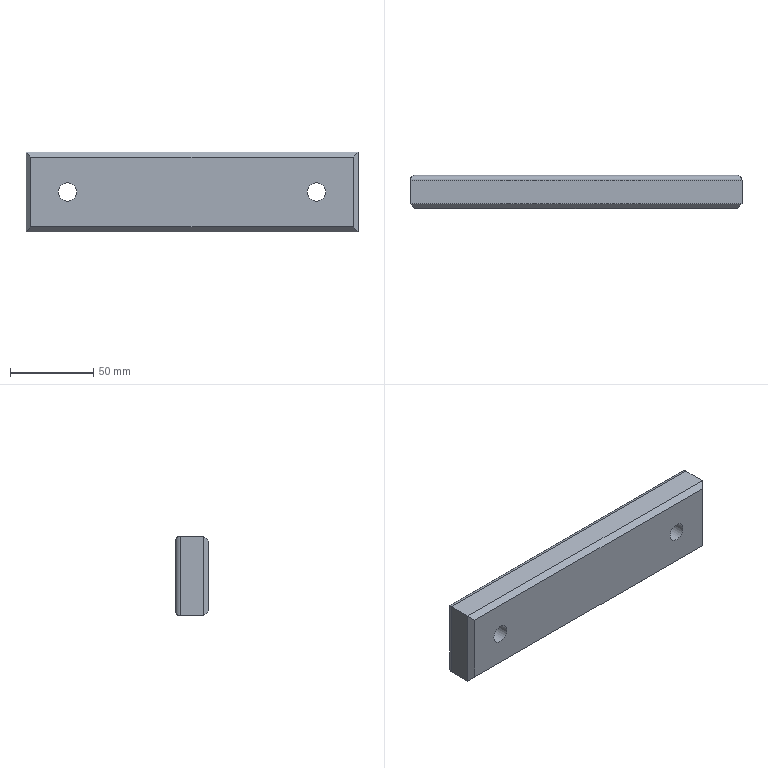Part | NX | features MAIN_BODY 2 | 1 solid | 20 faces | box 200 x 20 x 48 mm | volume 181563 mm3 | plane 12 | cylinder 8 | commonest cylinder face diameters 6 x4 11 x2 17.5 x2
STEP:
#1=CARTESIAN_POINT('',(95.,343.,-345.));
#2=VERTEX_POINT('',#1);
#3=CARTESIAN_POINT('',(95.,357.,-345.));
#4=VERTEX_POINT('',#3);
#5=CARTESIAN_POINT('',(95.,340.,-345.));
#6=DIRECTION('',(0.,1.,0.));
#7=VECTOR('',#6,1000.);
#8=LINE('',#5,#7);
#9=EDGE_CURVE('',#2,#4,#8,.T.);
#10=ORIENTED_EDGE('',*,*,#9,.F.);
#11=CARTESIAN_POINT('',(95.,343.,-297.));
#12=VERTEX_POINT('',#11);
#13=CARTESIAN_POINT('',(95.,343.,-297.));
#14=DIRECTION('',(0.,0.,1.));
#15=VECTOR('',#14,1000.);
#16=LINE('',#13,#15);
#17=EDGE_CURVE('',#2,#12,#16,.T.);
#18=ORIENTED_EDGE('',*,*,#17,.T.);
#19=CARTESIAN_POINT('',(95.,357.,-297.));
#20=VERTEX_POINT('',#19);
#21=CARTESIAN_POINT('',(95.,340.,-297.));
#22=DIRECTION('',(0.,1.,0.));
#23=VECTOR('',#22,1000.);
#24=LINE('',#21,#23);
#25=EDGE_CURVE('',#12,#20,#24,.T.);
#26=ORIENTED_EDGE('',*,*,#25,.T.);
#27=CARTESIAN_POINT('',(95.,357.,-297.));
#28=DIRECTION('',(0.,0.,-1.));
#29=VECTOR('',#28,1000.);
#30=LINE('',#27,#29);
#31=EDGE_CURVE('',#20,#4,#30,.T.);
#32=ORIENTED_EDGE('',*,*,#31,.T.);
#33=EDGE_LOOP('',(#10,#18,#26,#32));
#34=FACE_BOUND('',#33,.T.);
#35=CARTESIAN_POINT('',(95.,340.,-297.));
#36=DIRECTION('',(1.,0.,0.));
#37=DIRECTION('',(0.,1.,0.));
#38=AXIS2_PLACEMENT_3D('',#35,#36,#37);
#39=PLANE('',#38);
#40=ADVANCED_FACE('',(#34),#39,.F.);
#41=CARTESIAN_POINT('',(295.,343.,-345.));
#42=VERTEX_POINT('',#41);
#43=CARTESIAN_POINT('',(295.,357.,-345.));
#44=VERTEX_POINT('',#43);
#45=CARTESIAN_POINT('',(295.,340.,-345.));
#46=DIRECTION('',(0.,1.,0.));
#47=VECTOR('',#46,1000.);
#48=LINE('',#45,#47);
#49=EDGE_CURVE('',#42,#44,#48,.T.);
#50=ORIENTED_EDGE('',*,*,#49,.F.);
#51=CARTESIAN_POINT('',(95.,343.,-345.));
#52=DIRECTION('',(-1.,0.,0.));
#53=VECTOR('',#52,1000.);
#54=LINE('',#51,#53);
#55=EDGE_CURVE('',#42,#2,#54,.T.);
#56=ORIENTED_EDGE('',*,*,#55,.T.);
#57=ORIENTED_EDGE('',*,*,#9,.T.);
#58=CARTESIAN_POINT('',(95.,357.,-345.));
#59=DIRECTION('',(1.,0.,0.));
#60=VECTOR('',#59,1000.);
#61=LINE('',#58,#60);
#62=EDGE_CURVE('',#4,#44,#61,.T.);
#63=ORIENTED_EDGE('',*,*,#62,.T.);
#64=EDGE_LOOP('',(#50,#56,#57,#63));
#65=FACE_BOUND('',#64,.T.);
#66=CARTESIAN_POINT('',(95.,340.,-345.));
#67=DIRECTION('',(0.,0.,1.));
#68=DIRECTION('',(-1.,0.,0.));
#69=AXIS2_PLACEMENT_3D('',#66,#67,#68);
#70=PLANE('',#69);
#71=ADVANCED_FACE('',(#65),#70,.F.);
#72=CARTESIAN_POINT('',(295.,343.,-297.));
#73=VERTEX_POINT('',#72);
#74=CARTESIAN_POINT('',(295.,357.,-297.));
#75=VERTEX_POINT('',#74);
#76=CARTESIAN_POINT('',(295.,340.,-297.));
#77=DIRECTION('',(0.,1.,0.));
#78=VECTOR('',#77,1000.);
#79=LINE('',#76,#78);
#80=EDGE_CURVE('',#73,#75,#79,.T.);
#81=ORIENTED_EDGE('',*,*,#80,.F.);
#82=CARTESIAN_POINT('',(295.,343.,-345.));
#83=DIRECTION('',(0.,0.,-1.));
#84=VECTOR('',#83,1000.);
#85=LINE('',#82,#84);
#86=EDGE_CURVE('',#73,#42,#85,.T.);
#87=ORIENTED_EDGE('',*,*,#86,.T.);
#88=ORIENTED_EDGE('',*,*,#49,.T.);
#89=CARTESIAN_POINT('',(295.,357.,-345.));
#90=DIRECTION('',(0.,0.,1.));
#91=VECTOR('',#90,1000.);
#92=LINE('',#89,#91);
#93=EDGE_CURVE('',#44,#75,#92,.T.);
#94=ORIENTED_EDGE('',*,*,#93,.T.);
#95=EDGE_LOOP('',(#81,#87,#88,#94));
#96=FACE_BOUND('',#95,.T.);
#97=CARTESIAN_POINT('',(295.,340.,-345.));
#98=DIRECTION('',(-1.,0.,0.));
#99=DIRECTION('',(0.,-1.,0.));
#100=AXIS2_PLACEMENT_3D('',#97,#98,#99);
#101=PLANE('',#100);
#102=ADVANCED_FACE('',(#96),#101,.F.);
#103=ORIENTED_EDGE('',*,*,#25,.F.);
#104=CARTESIAN_POINT('',(295.,343.,-297.));
#105=DIRECTION('',(1.,0.,0.));
#106=VECTOR('',#105,1000.);
#107=LINE('',#104,#106);
#108=EDGE_CURVE('',#12,#73,#107,.T.);
#109=ORIENTED_EDGE('',*,*,#108,.T.);
#110=ORIENTED_EDGE('',*,*,#80,.T.);
#111=CARTESIAN_POINT('',(295.,357.,-297.));
#112=DIRECTION('',(-1.,0.,0.));
#113=VECTOR('',#112,1000.);
#114=LINE('',#111,#113);
#115=EDGE_CURVE('',#75,#20,#114,.T.);
#116=ORIENTED_EDGE('',*,*,#115,.T.);
#117=EDGE_LOOP('',(#103,#109,#110,#116));
#118=FACE_BOUND('',#117,.T.);
#119=CARTESIAN_POINT('',(295.,340.,-297.));
#120=DIRECTION('',(0.,0.,-1.));
#121=DIRECTION('',(1.,0.,0.));
#122=AXIS2_PLACEMENT_3D('',#119,#120,#121);
#123=PLANE('',#122);
#124=ADVANCED_FACE('',(#118),#123,.F.);
#125=CARTESIAN_POINT('',(98.,340.,-342.));
#126=VERTEX_POINT('',#125);
#127=CARTESIAN_POINT('',(292.,340.,-342.));
#128=VERTEX_POINT('',#127);
#129=CARTESIAN_POINT('',(295.,340.,-342.));
#130=DIRECTION('',(1.,0.,0.));
#131=VECTOR('',#130,1000.);
#132=LINE('',#129,#131);
#133=EDGE_CURVE('',#126,#128,#132,.T.);
#134=ORIENTED_EDGE('',*,*,#133,.T.);
#135=CARTESIAN_POINT('',(292.,340.,-300.));
#136=VERTEX_POINT('',#135);
#137=CARTESIAN_POINT('',(292.,340.,-297.));
#138=DIRECTION('',(0.,0.,1.));
#139=VECTOR('',#138,1000.);
#140=LINE('',#137,#139);
#141=EDGE_CURVE('',#128,#136,#140,.T.);
#142=ORIENTED_EDGE('',*,*,#141,.T.);
#143=CARTESIAN_POINT('',(98.,340.,-300.));
#144=VERTEX_POINT('',#143);
#145=CARTESIAN_POINT('',(95.,340.,-300.));
#146=DIRECTION('',(-1.,0.,0.));
#147=VECTOR('',#146,1000.);
#148=LINE('',#145,#147);
#149=EDGE_CURVE('',#136,#144,#148,.T.);
#150=ORIENTED_EDGE('',*,*,#149,.T.);
#151=CARTESIAN_POINT('',(98.,340.,-345.));
#152=DIRECTION('',(0.,0.,-1.));
#153=VECTOR('',#152,1000.);
#154=LINE('',#151,#153);
#155=EDGE_CURVE('',#144,#126,#154,.T.);
#156=ORIENTED_EDGE('',*,*,#155,.T.);
#157=EDGE_LOOP('',(#134,#142,#150,#156));
#158=FACE_BOUND('',#157,.T.);
#159=CARTESIAN_POINT('',(275.5,340.,-321.));
#160=VERTEX_POINT('',#159);
#161=CARTESIAN_POINT('',(270.,340.,-321.));
#162=DIRECTION('',(0.,-1.,0.));
#163=DIRECTION('',(1.,0.,0.));
#164=AXIS2_PLACEMENT_3D('',#161,#162,#163);
#165=CIRCLE('',#164,5.5);
#166=EDGE_CURVE('',#160,#160,#165,.T.);
#167=ORIENTED_EDGE('',*,*,#166,.F.);
#168=EDGE_LOOP('',(#167));
#169=FACE_BOUND('',#168,.T.);
#170=CARTESIAN_POINT('',(125.5,340.,-321.));
#171=VERTEX_POINT('',#170);
#172=CARTESIAN_POINT('',(120.,340.,-321.));
#173=DIRECTION('',(0.,-1.,0.));
#174=DIRECTION('',(1.,0.,0.));
#175=AXIS2_PLACEMENT_3D('',#172,#173,#174);
#176=CIRCLE('',#175,5.5);
#177=EDGE_CURVE('',#171,#171,#176,.T.);
#178=ORIENTED_EDGE('',*,*,#177,.F.);
#179=EDGE_LOOP('',(#178));
#180=FACE_BOUND('',#179,.T.);
#181=CARTESIAN_POINT('',(95.,340.,-345.));
#182=DIRECTION('',(0.,-1.,0.));
#183=DIRECTION('',(1.,0.,0.));
#184=AXIS2_PLACEMENT_3D('',#181,#182,#183);
#185=PLANE('',#184);
#186=ADVANCED_FACE('',(#158,#169,#180),#185,.T.);
#187=CARTESIAN_POINT('',(98.,360.,-342.));
#188=VERTEX_POINT('',#187);
#189=CARTESIAN_POINT('',(98.,360.,-300.));
#190=VERTEX_POINT('',#189);
#191=CARTESIAN_POINT('',(98.,360.,-345.));
#192=DIRECTION('',(0.,0.,-1.));
#193=VECTOR('',#192,1000.);
#194=LINE('',#191,#193);
#195=EDGE_CURVE('',#188,#190,#194,.F.);
#196=ORIENTED_EDGE('',*,*,#195,.T.);
#197=CARTESIAN_POINT('',(292.,360.,-300.));
#198=VERTEX_POINT('',#197);
#199=CARTESIAN_POINT('',(95.,360.,-300.));
#200=DIRECTION('',(-1.,0.,0.));
#201=VECTOR('',#200,1000.);
#202=LINE('',#199,#201);
#203=EDGE_CURVE('',#190,#198,#202,.F.);
#204=ORIENTED_EDGE('',*,*,#203,.T.);
#205=CARTESIAN_POINT('',(292.,360.,-342.));
#206=VERTEX_POINT('',#205);
#207=CARTESIAN_POINT('',(292.,360.,-345.));
#208=DIRECTION('',(0.,0.,1.));
#209=VECTOR('',#208,1000.);
#210=LINE('',#207,#209);
#211=EDGE_CURVE('',#198,#206,#210,.F.);
#212=ORIENTED_EDGE('',*,*,#211,.T.);
#213=CARTESIAN_POINT('',(95.,360.,-342.));
#214=DIRECTION('',(1.,0.,0.));
#215=VECTOR('',#214,1000.);
#216=LINE('',#213,#215);
#217=EDGE_CURVE('',#206,#188,#216,.F.);
#218=ORIENTED_EDGE('',*,*,#217,.T.);
#219=EDGE_LOOP('',(#196,#204,#212,#218));
#220=FACE_BOUND('',#219,.T.);
#221=CARTESIAN_POINT('',(278.75,360.,-321.));
#222=VERTEX_POINT('',#221);
#223=CARTESIAN_POINT('',(270.,360.,-321.));
#224=DIRECTION('',(0.,-1.,0.));
#225=DIRECTION('',(1.,0.,0.));
#226=AXIS2_PLACEMENT_3D('',#223,#224,#225);
#227=CIRCLE('',#226,8.75);
#228=EDGE_CURVE('',#222,#222,#227,.T.);
#229=ORIENTED_EDGE('',*,*,#228,.T.);
#230=EDGE_LOOP('',(#229));
#231=FACE_BOUND('',#230,.T.);
#232=CARTESIAN_POINT('',(128.75,360.,-321.));
#233=VERTEX_POINT('',#232);
#234=CARTESIAN_POINT('',(120.,360.,-321.));
#235=DIRECTION('',(0.,-1.,0.));
#236=DIRECTION('',(1.,0.,0.));
#237=AXIS2_PLACEMENT_3D('',#234,#235,#236);
#238=CIRCLE('',#237,8.75);
#239=EDGE_CURVE('',#233,#233,#238,.T.);
#240=ORIENTED_EDGE('',*,*,#239,.T.);
#241=EDGE_LOOP('',(#240));
#242=FACE_BOUND('',#241,.T.);
#243=CARTESIAN_POINT('',(95.,360.,-345.));
#244=DIRECTION('',(0.,-1.,0.));
#245=DIRECTION('',(1.,0.,0.));
#246=AXIS2_PLACEMENT_3D('',#243,#244,#245);
#247=PLANE('',#246);
#248=ADVANCED_FACE('',(#220,#231,#242),#247,.F.);
#249=ORIENTED_EDGE('',*,*,#177,.T.);
#250=EDGE_LOOP('',(#249));
#251=FACE_BOUND('',#250,.T.);
#252=CARTESIAN_POINT('',(125.5,348.,-321.));
#253=VERTEX_POINT('',#252);
#254=CARTESIAN_POINT('',(120.,348.,-321.));
#255=DIRECTION('',(0.,-1.,0.));
#256=DIRECTION('',(1.,0.,0.));
#257=AXIS2_PLACEMENT_3D('',#254,#255,#256);
#258=CIRCLE('',#257,5.5);
#259=EDGE_CURVE('',#253,#253,#258,.T.);
#260=ORIENTED_EDGE('',*,*,#259,.F.);
#261=EDGE_LOOP('',(#260));
#262=FACE_BOUND('',#261,.T.);
#263=CARTESIAN_POINT('',(120.,310.,-321.));
#264=DIRECTION('',(0.,-1.,0.));
#265=DIRECTION('',(1.,0.,0.));
#266=AXIS2_PLACEMENT_3D('',#263,#264,#265);
#267=CYLINDRICAL_SURFACE('',#266,5.5);
#268=ADVANCED_FACE('',(#251,#262),#267,.F.);
#269=ORIENTED_EDGE('',*,*,#259,.T.);
#270=EDGE_LOOP('',(#269));
#271=FACE_BOUND('',#270,.T.);
#272=CARTESIAN_POINT('',(128.75,348.,-321.));
#273=VERTEX_POINT('',#272);
#274=CARTESIAN_POINT('',(120.,348.,-321.));
#275=DIRECTION('',(0.,-1.,0.));
#276=DIRECTION('',(1.,0.,0.));
#277=AXIS2_PLACEMENT_3D('',#274,#275,#276);
#278=CIRCLE('',#277,8.75);
#279=EDGE_CURVE('',#273,#273,#278,.T.);
#280=ORIENTED_EDGE('',*,*,#279,.F.);
#281=EDGE_LOOP('',(#280));
#282=FACE_BOUND('',#281,.T.);
#283=CARTESIAN_POINT('',(120.,348.,-321.));
#284=DIRECTION('',(0.,-1.,0.));
#285=DIRECTION('',(1.,0.,0.));
#286=AXIS2_PLACEMENT_3D('',#283,#284,#285);
#287=PLANE('',#286);
#288=ADVANCED_FACE('',(#271,#282),#287,.F.);
#289=ORIENTED_EDGE('',*,*,#279,.T.);
#290=EDGE_LOOP('',(#289));
#291=FACE_BOUND('',#290,.T.);
#292=ORIENTED_EDGE('',*,*,#239,.F.);
#293=EDGE_LOOP('',(#292));
#294=FACE_BOUND('',#293,.T.);
#295=CARTESIAN_POINT('',(120.,360.,-321.));
#296=DIRECTION('',(0.,-1.,0.));
#297=DIRECTION('',(1.,0.,0.));
#298=AXIS2_PLACEMENT_3D('',#295,#296,#297);
#299=CYLINDRICAL_SURFACE('',#298,8.75);
#300=ADVANCED_FACE('',(#291,#294),#299,.F.);
#301=ORIENTED_EDGE('',*,*,#166,.T.);
#302=EDGE_LOOP('',(#301));
#303=FACE_BOUND('',#302,.T.);
#304=CARTESIAN_POINT('',(275.5,348.,-321.));
#305=VERTEX_POINT('',#304);
#306=CARTESIAN_POINT('',(270.,348.,-321.));
#307=DIRECTION('',(0.,-1.,0.));
#308=DIRECTION('',(1.,0.,0.));
#309=AXIS2_PLACEMENT_3D('',#306,#307,#308);
#310=CIRCLE('',#309,5.5);
#311=EDGE_CURVE('',#305,#305,#310,.T.);
#312=ORIENTED_EDGE('',*,*,#311,.F.);
#313=EDGE_LOOP('',(#312));
#314=FACE_BOUND('',#313,.T.);
#315=CARTESIAN_POINT('',(270.,310.,-321.));
#316=DIRECTION('',(0.,-1.,0.));
#317=DIRECTION('',(1.,0.,0.));
#318=AXIS2_PLACEMENT_3D('',#315,#316,#317);
#319=CYLINDRICAL_SURFACE('',#318,5.5);
#320=ADVANCED_FACE('',(#303,#314),#319,.F.);
#321=ORIENTED_EDGE('',*,*,#311,.T.);
#322=EDGE_LOOP('',(#321));
#323=FACE_BOUND('',#322,.T.);
#324=CARTESIAN_POINT('',(278.75,348.,-321.));
#325=VERTEX_POINT('',#324);
#326=CARTESIAN_POINT('',(270.,348.,-321.));
#327=DIRECTION('',(0.,-1.,0.));
#328=DIRECTION('',(1.,0.,0.));
#329=AXIS2_PLACEMENT_3D('',#326,#327,#328);
#330=CIRCLE('',#329,8.75);
#331=EDGE_CURVE('',#325,#325,#330,.T.);
#332=ORIENTED_EDGE('',*,*,#331,.F.);
#333=EDGE_LOOP('',(#332));
#334=FACE_BOUND('',#333,.T.);
#335=CARTESIAN_POINT('',(270.,348.,-321.));
#336=DIRECTION('',(0.,-1.,0.));
#337=DIRECTION('',(1.,0.,0.));
#338=AXIS2_PLACEMENT_3D('',#335,#336,#337);
#339=PLANE('',#338);
#340=ADVANCED_FACE('',(#323,#334),#339,.F.);
#341=ORIENTED_EDGE('',*,*,#331,.T.);
#342=EDGE_LOOP('',(#341));
#343=FACE_BOUND('',#342,.T.);
#344=ORIENTED_EDGE('',*,*,#228,.F.);
#345=EDGE_LOOP('',(#344));
#346=FACE_BOUND('',#345,.T.);
#347=CARTESIAN_POINT('',(270.,360.,-321.));
#348=DIRECTION('',(0.,-1.,0.));
#349=DIRECTION('',(1.,0.,0.));
#350=AXIS2_PLACEMENT_3D('',#347,#348,#349);
#351=CYLINDRICAL_SURFACE('',#350,8.75);
#352=ADVANCED_FACE('',(#343,#346),#351,.F.);
#353=CARTESIAN_POINT('',(98.,357.,-342.));
#354=DIRECTION('',(0.7071,0.,-0.7071));
#355=DIRECTION('',(-0.7071,0.,-0.7071));
#356=AXIS2_PLACEMENT_3D('',#353,#354,#355);
#357=ELLIPSE('',#356,4.243,3.);
#358=EDGE_CURVE('',#188,#4,#357,.F.);
#359=ORIENTED_EDGE('',*,*,#358,.F.);
#360=ORIENTED_EDGE('',*,*,#217,.F.);
#361=CARTESIAN_POINT('',(292.,357.,-342.));
#362=DIRECTION('',(0.7071,0.,0.7071));
#363=DIRECTION('',(0.7071,0.,-0.7071));
#364=AXIS2_PLACEMENT_3D('',#361,#362,#363);
#365=ELLIPSE('',#364,4.243,3.);
#366=EDGE_CURVE('',#44,#206,#365,.T.);
#367=ORIENTED_EDGE('',*,*,#366,.F.);
#368=ORIENTED_EDGE('',*,*,#62,.F.);
#369=EDGE_LOOP('',(#359,#360,#367,#368));
#370=FACE_BOUND('',#369,.T.);
#371=CARTESIAN_POINT('',(95.,357.,-342.));
#372=DIRECTION('',(1.,0.,0.));
#373=DIRECTION('',(0.,0.,1.));
#374=AXIS2_PLACEMENT_3D('',#371,#372,#373);
#375=CYLINDRICAL_SURFACE('',#374,3.);
#376=ADVANCED_FACE('',(#370),#375,.T.);
#377=ORIENTED_EDGE('',*,*,#366,.T.);
#378=ORIENTED_EDGE('',*,*,#211,.F.);
#379=CARTESIAN_POINT('',(292.,357.,-300.));
#380=DIRECTION('',(-0.7071,0.,0.7071));
#381=DIRECTION('',(0.7071,0.,0.7071));
#382=AXIS2_PLACEMENT_3D('',#379,#380,#381);
#383=ELLIPSE('',#382,4.243,3.);
#384=EDGE_CURVE('',#75,#198,#383,.T.);
#385=ORIENTED_EDGE('',*,*,#384,.F.);
#386=ORIENTED_EDGE('',*,*,#93,.F.);
#387=EDGE_LOOP('',(#377,#378,#385,#386));
#388=FACE_BOUND('',#387,.T.);
#389=CARTESIAN_POINT('',(292.,357.,-345.));
#390=DIRECTION('',(0.,0.,1.));
#391=DIRECTION('',(0.,-1.,0.));
#392=AXIS2_PLACEMENT_3D('',#389,#390,#391);
#393=CYLINDRICAL_SURFACE('',#392,3.);
#394=ADVANCED_FACE('',(#388),#393,.T.);
#395=ORIENTED_EDGE('',*,*,#358,.T.);
#396=ORIENTED_EDGE('',*,*,#31,.F.);
#397=CARTESIAN_POINT('',(98.,357.,-300.));
#398=DIRECTION('',(-0.7071,0.,-0.7071));
#399=DIRECTION('',(0.7071,0.,-0.7071));
#400=AXIS2_PLACEMENT_3D('',#397,#398,#399);
#401=ELLIPSE('',#400,4.243,3.);
#402=EDGE_CURVE('',#190,#20,#401,.F.);
#403=ORIENTED_EDGE('',*,*,#402,.F.);
#404=ORIENTED_EDGE('',*,*,#195,.F.);
#405=EDGE_LOOP('',(#395,#396,#403,#404));
#406=FACE_BOUND('',#405,.T.);
#407=CARTESIAN_POINT('',(98.,357.,-297.));
#408=DIRECTION('',(0.,0.,-1.));
#409=DIRECTION('',(0.,1.,0.));
#410=AXIS2_PLACEMENT_3D('',#407,#408,#409);
#411=CYLINDRICAL_SURFACE('',#410,3.);
#412=ADVANCED_FACE('',(#406),#411,.T.);
#413=ORIENTED_EDGE('',*,*,#384,.T.);
#414=ORIENTED_EDGE('',*,*,#203,.F.);
#415=ORIENTED_EDGE('',*,*,#402,.T.);
#416=ORIENTED_EDGE('',*,*,#115,.F.);
#417=EDGE_LOOP('',(#413,#414,#415,#416));
#418=FACE_BOUND('',#417,.T.);
#419=CARTESIAN_POINT('',(295.,357.,-300.));
#420=DIRECTION('',(-1.,0.,0.));
#421=DIRECTION('',(0.,0.,-1.));
#422=AXIS2_PLACEMENT_3D('',#419,#420,#421);
#423=CYLINDRICAL_SURFACE('',#422,3.);
#424=ADVANCED_FACE('',(#418),#423,.T.);
#425=CARTESIAN_POINT('',(97.,341.,-299.));
#426=DIRECTION('',(0.5774,-0.5774,-0.5774));
#427=VECTOR('',#426,1000.);
#428=LINE('',#425,#427);
#429=EDGE_CURVE('',#12,#144,#428,.T.);
#430=ORIENTED_EDGE('',*,*,#429,.F.);
#431=ORIENTED_EDGE('',*,*,#17,.F.);
#432=CARTESIAN_POINT('',(97.,341.,-343.));
#433=DIRECTION('',(0.5774,-0.5774,0.5774));
#434=VECTOR('',#433,1000.);
#435=LINE('',#432,#434);
#436=EDGE_CURVE('',#126,#2,#435,.F.);
#437=ORIENTED_EDGE('',*,*,#436,.F.);
#438=ORIENTED_EDGE('',*,*,#155,.F.);
#439=EDGE_LOOP('',(#430,#431,#437,#438));
#440=FACE_BOUND('',#439,.T.);
#441=CARTESIAN_POINT('',(98.,340.,-345.));
#442=DIRECTION('',(-0.7071,-0.7071,0.));
#443=DIRECTION('',(0.7071,-0.7071,0.));
#444=AXIS2_PLACEMENT_3D('',#441,#442,#443);
#445=PLANE('',#444);
#446=ADVANCED_FACE('',(#440),#445,.T.);
#447=ORIENTED_EDGE('',*,*,#436,.T.);
#448=ORIENTED_EDGE('',*,*,#55,.F.);
#449=CARTESIAN_POINT('',(226.333,274.333,-276.333));
#450=DIRECTION('',(-0.5774,-0.5774,0.5774));
#451=VECTOR('',#450,1000.);
#452=LINE('',#449,#451);
#453=EDGE_CURVE('',#128,#42,#452,.F.);
#454=ORIENTED_EDGE('',*,*,#453,.F.);
#455=ORIENTED_EDGE('',*,*,#133,.F.);
#456=EDGE_LOOP('',(#447,#448,#454,#455));
#457=FACE_BOUND('',#456,.T.);
#458=CARTESIAN_POINT('',(95.,340.,-342.));
#459=DIRECTION('',(0.,-0.7071,-0.7071));
#460=DIRECTION('',(0.,0.7071,-0.7071));
#461=AXIS2_PLACEMENT_3D('',#458,#459,#460);
#462=PLANE('',#461);
#463=ADVANCED_FACE('',(#457),#462,.T.);
#464=ORIENTED_EDGE('',*,*,#429,.T.);
#465=ORIENTED_EDGE('',*,*,#149,.F.);
#466=CARTESIAN_POINT('',(226.333,274.333,-365.667));
#467=DIRECTION('',(0.5774,0.5774,0.5774));
#468=VECTOR('',#467,1000.);
#469=LINE('',#466,#468);
#470=EDGE_CURVE('',#73,#136,#469,.F.);
#471=ORIENTED_EDGE('',*,*,#470,.F.);
#472=ORIENTED_EDGE('',*,*,#108,.F.);
#473=EDGE_LOOP('',(#464,#465,#471,#472));
#474=FACE_BOUND('',#473,.T.);
#475=CARTESIAN_POINT('',(95.,340.,-300.));
#476=DIRECTION('',(0.,-0.7071,0.7071));
#477=DIRECTION('',(0.,-0.7071,-0.7071));
#478=AXIS2_PLACEMENT_3D('',#475,#476,#477);
#479=PLANE('',#478);
#480=ADVANCED_FACE('',(#474),#479,.T.);
#481=ORIENTED_EDGE('',*,*,#453,.T.);
#482=ORIENTED_EDGE('',*,*,#86,.F.);
#483=ORIENTED_EDGE('',*,*,#470,.T.);
#484=ORIENTED_EDGE('',*,*,#141,.F.);
#485=EDGE_LOOP('',(#481,#482,#483,#484));
#486=FACE_BOUND('',#485,.T.);
#487=CARTESIAN_POINT('',(292.,340.,-345.));
#488=DIRECTION('',(0.7071,-0.7071,0.));
#489=DIRECTION('',(0.7071,0.7071,0.));
#490=AXIS2_PLACEMENT_3D('',#487,#488,#489);
#491=PLANE('',#490);
#492=ADVANCED_FACE('',(#486),#491,.T.);
#493=CLOSED_SHELL('',(#40,#71,#102,#124,#186,#248,#268,#288,#300,#320,#340,#352,#376,#394,#412,#424,#446,#463,#480,#492));
#494=MANIFOLD_SOLID_BREP('',#493);
#495=(LENGTH_UNIT()NAMED_UNIT(*)SI_UNIT(.MILLI.,.METRE.));
#496=UNCERTAINTY_MEASURE_WITH_UNIT(LENGTH_MEASURE(0.00001),#495,'','');
#497=(NAMED_UNIT(*)PLANE_ANGLE_UNIT()SI_UNIT($,.RADIAN.));
#498=(NAMED_UNIT(*)SI_UNIT($,.STERADIAN.)SOLID_ANGLE_UNIT());
#499=(GEOMETRIC_REPRESENTATION_CONTEXT(3)GLOBAL_UNCERTAINTY_ASSIGNED_CONTEXT((#496))GLOBAL_UNIT_ASSIGNED_CONTEXT((#495,#497,#498))REPRESENTATION_CONTEXT('',''));
#500=ADVANCED_BREP_SHAPE_REPRESENTATION('',(#494),#499);